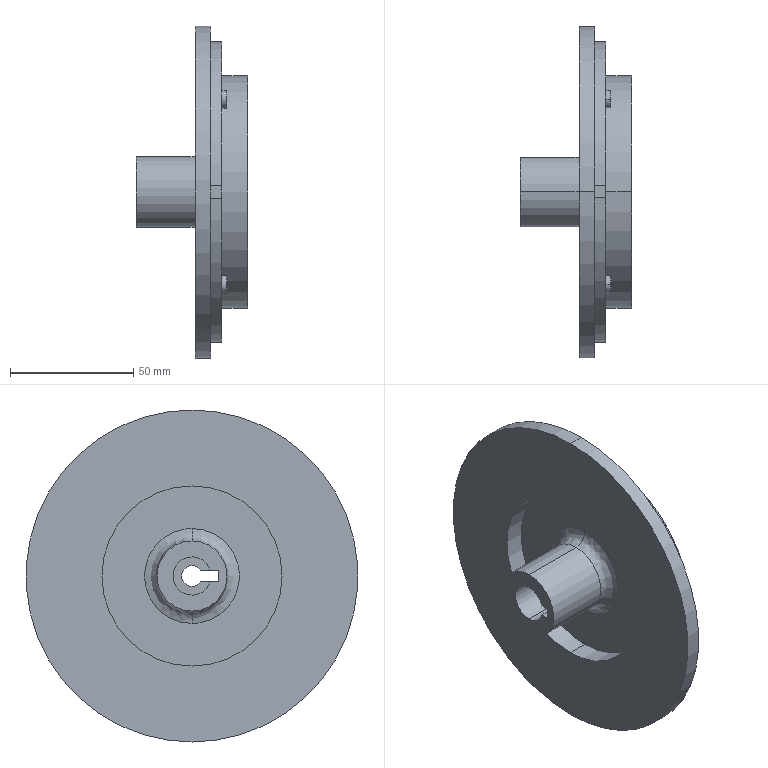Part | STEP file | 10P30 hub | 1 solid | 60 faces | box 45 x 134.5 x 134.5 mm | volume 158986 mm3 | cylinder 30 | plane 28 | spline 2 | commonest cylinder face diameters 7 x8 122 x4 8.5 x3 15.5 x3 22 x2 28.4 x2